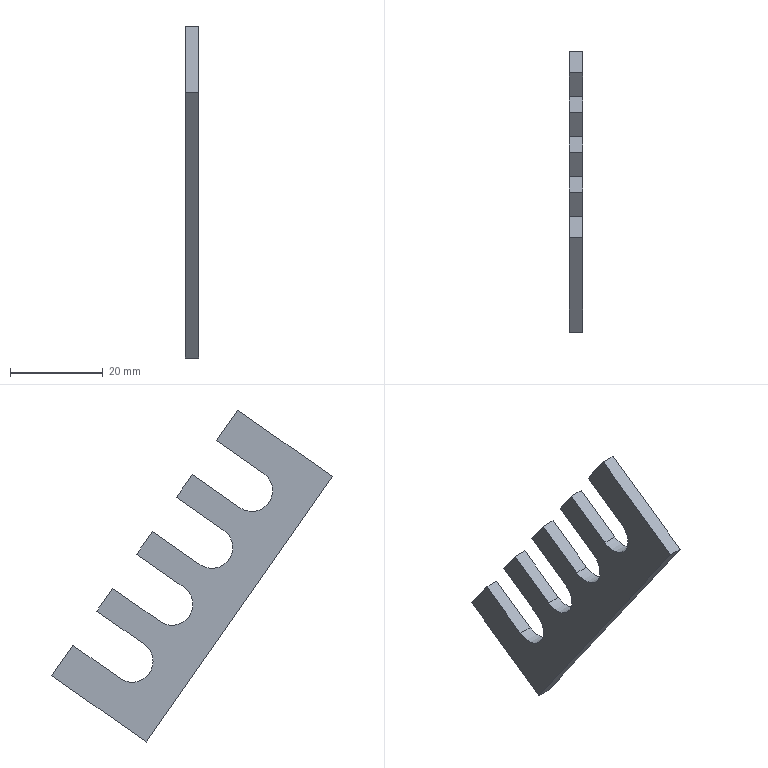Part | STEP file | Positioning_id1774_x_t | 1 solid | 22 faces | box 3 x 60.629 x 71.68 mm | volume 3518 mm3 | plane 18 | cylinder 4 | commonest cylinder face diameters 9 x4